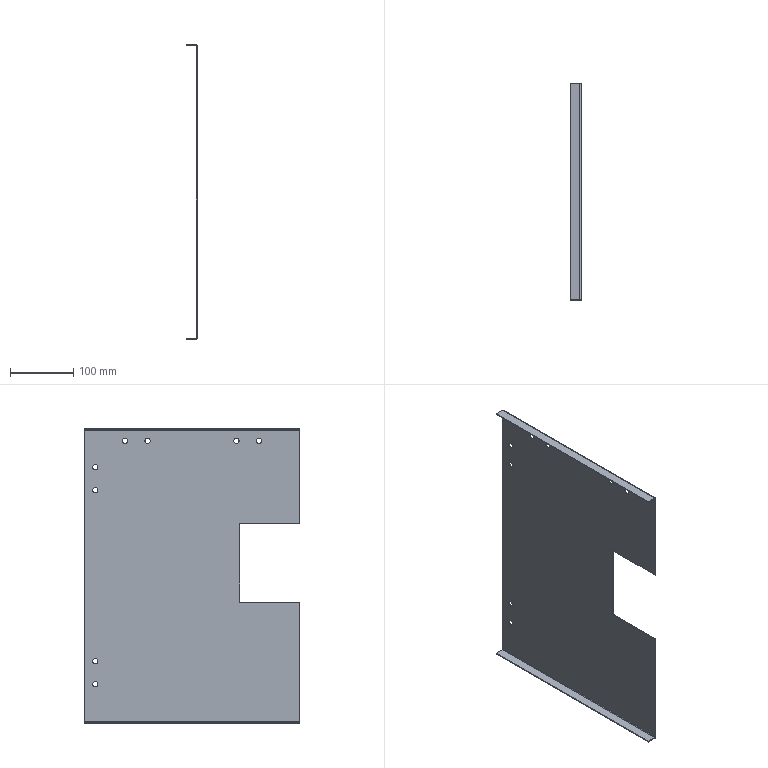Part | SolidWorks | features BaseBody 1 | 1 solid | 34 faces | box 16.5 x 340 x 464 mm | volume 232938 mm3 | cylinder 20 | plane 14 | commonest cylinder face diameters 8.5 x16 1.473 x2 4.473 x2
STEP:
#1=CARTESIAN_POINT('',(0.,276.,-13.25));
#2=VERTEX_POINT('',#1);
#3=CARTESIAN_POINT('',(0.,276.,-21.75));
#4=VERTEX_POINT('',#3);
#5=CARTESIAN_POINT('',(0.,276.,-17.5));
#6=DIRECTION('',(1.,0.,0.));
#7=DIRECTION('',(0.,0.,-1.));
#8=AXIS2_PLACEMENT_3D('',#5,#6,#7);
#9=CIRCLE('',#8,4.25);
#10=EDGE_CURVE('',#2,#4,#9,.T.);
#11=ORIENTED_EDGE('',*,*,#10,.F.);
#12=CARTESIAN_POINT('',(1.5,276.,-13.25));
#13=VERTEX_POINT('',#12);
#14=CARTESIAN_POINT('',(-8.5,276.,-13.25));
#15=DIRECTION('',(1.,0.,0.));
#16=VECTOR('',#15,1000.);
#17=LINE('',#14,#16);
#18=EDGE_CURVE('',#2,#13,#17,.T.);
#19=ORIENTED_EDGE('',*,*,#18,.T.);
#20=CARTESIAN_POINT('',(1.5,276.,-21.75));
#21=VERTEX_POINT('',#20);
#22=CARTESIAN_POINT('',(1.5,276.,-17.5));
#23=DIRECTION('',(-1.,0.,0.));
#24=DIRECTION('',(0.,0.,-1.));
#25=AXIS2_PLACEMENT_3D('',#22,#23,#24);
#26=CIRCLE('',#25,4.25);
#27=EDGE_CURVE('',#21,#13,#26,.T.);
#28=ORIENTED_EDGE('',*,*,#27,.F.);
#29=CARTESIAN_POINT('',(-8.5,276.,-21.75));
#30=DIRECTION('',(1.,0.,0.));
#31=VECTOR('',#30,1000.);
#32=LINE('',#29,#31);
#33=EDGE_CURVE('',#4,#21,#32,.T.);
#34=ORIENTED_EDGE('',*,*,#33,.F.);
#35=EDGE_LOOP('',(#11,#19,#28,#34));
#36=FACE_OUTER_BOUND('',#35,.T.);
#37=CARTESIAN_POINT('',(-8.5,276.,-17.5));
#38=DIRECTION('',(1.,0.,0.));
#39=DIRECTION('',(0.,0.,-1.));
#40=AXIS2_PLACEMENT_3D('',#37,#38,#39);
#41=CYLINDRICAL_SURFACE('',#40,4.25);
#42=ADVANCED_FACE('',(#36),#41,.F.);
#43=CARTESIAN_POINT('',(0.,322.5,-396.75));
#44=VERTEX_POINT('',#43);
#45=CARTESIAN_POINT('',(0.,322.5,-405.25));
#46=VERTEX_POINT('',#45);
#47=CARTESIAN_POINT('',(0.,322.5,-401.));
#48=DIRECTION('',(1.,0.,0.));
#49=DIRECTION('',(0.,0.,-1.));
#50=AXIS2_PLACEMENT_3D('',#47,#48,#49);
#51=CIRCLE('',#50,4.25);
#52=EDGE_CURVE('',#44,#46,#51,.T.);
#53=ORIENTED_EDGE('',*,*,#52,.F.);
#54=CARTESIAN_POINT('',(1.5,322.5,-396.75));
#55=VERTEX_POINT('',#54);
#56=CARTESIAN_POINT('',(-8.5,322.5,-396.75));
#57=DIRECTION('',(1.,0.,0.));
#58=VECTOR('',#57,1000.);
#59=LINE('',#56,#58);
#60=EDGE_CURVE('',#44,#55,#59,.T.);
#61=ORIENTED_EDGE('',*,*,#60,.T.);
#62=CARTESIAN_POINT('',(1.5,322.5,-405.25));
#63=VERTEX_POINT('',#62);
#64=CARTESIAN_POINT('',(1.5,322.5,-401.));
#65=DIRECTION('',(-1.,0.,0.));
#66=DIRECTION('',(0.,0.,-1.));
#67=AXIS2_PLACEMENT_3D('',#64,#65,#66);
#68=CIRCLE('',#67,4.25);
#69=EDGE_CURVE('',#63,#55,#68,.T.);
#70=ORIENTED_EDGE('',*,*,#69,.F.);
#71=CARTESIAN_POINT('',(-8.5,322.5,-405.25));
#72=DIRECTION('',(1.,0.,0.));
#73=VECTOR('',#72,1000.);
#74=LINE('',#71,#73);
#75=EDGE_CURVE('',#46,#63,#74,.T.);
#76=ORIENTED_EDGE('',*,*,#75,.F.);
#77=EDGE_LOOP('',(#53,#61,#70,#76));
#78=FACE_OUTER_BOUND('',#77,.T.);
#79=CARTESIAN_POINT('',(-8.5,322.5,-401.));
#80=DIRECTION('',(1.,0.,0.));
#81=DIRECTION('',(0.,0.,-1.));
#82=AXIS2_PLACEMENT_3D('',#79,#80,#81);
#83=CYLINDRICAL_SURFACE('',#82,4.25);
#84=ADVANCED_FACE('',(#78),#83,.F.);
#85=CARTESIAN_POINT('',(0.,322.5,-360.75));
#86=VERTEX_POINT('',#85);
#87=CARTESIAN_POINT('',(0.,322.5,-369.25));
#88=VERTEX_POINT('',#87);
#89=CARTESIAN_POINT('',(0.,322.5,-365.));
#90=DIRECTION('',(1.,0.,0.));
#91=DIRECTION('',(0.,0.,-1.));
#92=AXIS2_PLACEMENT_3D('',#89,#90,#91);
#93=CIRCLE('',#92,4.25);
#94=EDGE_CURVE('',#86,#88,#93,.T.);
#95=ORIENTED_EDGE('',*,*,#94,.F.);
#96=CARTESIAN_POINT('',(1.5,322.5,-360.75));
#97=VERTEX_POINT('',#96);
#98=CARTESIAN_POINT('',(-8.5,322.5,-360.75));
#99=DIRECTION('',(1.,0.,0.));
#100=VECTOR('',#99,1000.);
#101=LINE('',#98,#100);
#102=EDGE_CURVE('',#86,#97,#101,.T.);
#103=ORIENTED_EDGE('',*,*,#102,.T.);
#104=CARTESIAN_POINT('',(1.5,322.5,-369.25));
#105=VERTEX_POINT('',#104);
#106=CARTESIAN_POINT('',(1.5,322.5,-365.));
#107=DIRECTION('',(-1.,0.,0.));
#108=DIRECTION('',(0.,0.,-1.));
#109=AXIS2_PLACEMENT_3D('',#106,#107,#108);
#110=CIRCLE('',#109,4.25);
#111=EDGE_CURVE('',#105,#97,#110,.T.);
#112=ORIENTED_EDGE('',*,*,#111,.F.);
#113=CARTESIAN_POINT('',(-8.5,322.5,-369.25));
#114=DIRECTION('',(1.,0.,0.));
#115=VECTOR('',#114,1000.);
#116=LINE('',#113,#115);
#117=EDGE_CURVE('',#88,#105,#116,.T.);
#118=ORIENTED_EDGE('',*,*,#117,.F.);
#119=EDGE_LOOP('',(#95,#103,#112,#118));
#120=FACE_OUTER_BOUND('',#119,.T.);
#121=CARTESIAN_POINT('',(-8.5,322.5,-365.));
#122=DIRECTION('',(1.,0.,0.));
#123=DIRECTION('',(0.,0.,-1.));
#124=AXIS2_PLACEMENT_3D('',#121,#122,#123);
#125=CYLINDRICAL_SURFACE('',#124,4.25);
#126=ADVANCED_FACE('',(#120),#125,.F.);
#127=CARTESIAN_POINT('',(0.,322.5,-54.75));
#128=VERTEX_POINT('',#127);
#129=CARTESIAN_POINT('',(0.,322.5,-63.25));
#130=VERTEX_POINT('',#129);
#131=CARTESIAN_POINT('',(0.,322.5,-59.));
#132=DIRECTION('',(1.,0.,0.));
#133=DIRECTION('',(0.,0.,-1.));
#134=AXIS2_PLACEMENT_3D('',#131,#132,#133);
#135=CIRCLE('',#134,4.25);
#136=EDGE_CURVE('',#128,#130,#135,.T.);
#137=ORIENTED_EDGE('',*,*,#136,.F.);
#138=CARTESIAN_POINT('',(1.5,322.5,-54.75));
#139=VERTEX_POINT('',#138);
#140=CARTESIAN_POINT('',(-8.5,322.5,-54.75));
#141=DIRECTION('',(1.,0.,0.));
#142=VECTOR('',#141,1000.);
#143=LINE('',#140,#142);
#144=EDGE_CURVE('',#128,#139,#143,.T.);
#145=ORIENTED_EDGE('',*,*,#144,.T.);
#146=CARTESIAN_POINT('',(1.5,322.5,-63.25));
#147=VERTEX_POINT('',#146);
#148=CARTESIAN_POINT('',(1.5,322.5,-59.));
#149=DIRECTION('',(-1.,0.,0.));
#150=DIRECTION('',(0.,0.,-1.));
#151=AXIS2_PLACEMENT_3D('',#148,#149,#150);
#152=CIRCLE('',#151,4.25);
#153=EDGE_CURVE('',#147,#139,#152,.T.);
#154=ORIENTED_EDGE('',*,*,#153,.F.);
#155=CARTESIAN_POINT('',(-8.5,322.5,-63.25));
#156=DIRECTION('',(1.,0.,0.));
#157=VECTOR('',#156,1000.);
#158=LINE('',#155,#157);
#159=EDGE_CURVE('',#130,#147,#158,.T.);
#160=ORIENTED_EDGE('',*,*,#159,.F.);
#161=EDGE_LOOP('',(#137,#145,#154,#160));
#162=FACE_OUTER_BOUND('',#161,.T.);
#163=CARTESIAN_POINT('',(-8.5,322.5,-59.));
#164=DIRECTION('',(1.,0.,0.));
#165=DIRECTION('',(0.,0.,-1.));
#166=AXIS2_PLACEMENT_3D('',#163,#164,#165);
#167=CYLINDRICAL_SURFACE('',#166,4.25);
#168=ADVANCED_FACE('',(#162),#167,.F.);
#169=CARTESIAN_POINT('',(0.,322.5,-90.75));
#170=VERTEX_POINT('',#169);
#171=CARTESIAN_POINT('',(0.,322.5,-99.25));
#172=VERTEX_POINT('',#171);
#173=CARTESIAN_POINT('',(0.,322.5,-95.));
#174=DIRECTION('',(1.,0.,0.));
#175=DIRECTION('',(0.,0.,-1.));
#176=AXIS2_PLACEMENT_3D('',#173,#174,#175);
#177=CIRCLE('',#176,4.25);
#178=EDGE_CURVE('',#170,#172,#177,.T.);
#179=ORIENTED_EDGE('',*,*,#178,.F.);
#180=CARTESIAN_POINT('',(1.5,322.5,-90.75));
#181=VERTEX_POINT('',#180);
#182=CARTESIAN_POINT('',(-8.5,322.5,-90.75));
#183=DIRECTION('',(1.,0.,0.));
#184=VECTOR('',#183,1000.);
#185=LINE('',#182,#184);
#186=EDGE_CURVE('',#170,#181,#185,.T.);
#187=ORIENTED_EDGE('',*,*,#186,.T.);
#188=CARTESIAN_POINT('',(1.5,322.5,-99.25));
#189=VERTEX_POINT('',#188);
#190=CARTESIAN_POINT('',(1.5,322.5,-95.));
#191=DIRECTION('',(-1.,0.,0.));
#192=DIRECTION('',(0.,0.,-1.));
#193=AXIS2_PLACEMENT_3D('',#190,#191,#192);
#194=CIRCLE('',#193,4.25);
#195=EDGE_CURVE('',#189,#181,#194,.T.);
#196=ORIENTED_EDGE('',*,*,#195,.F.);
#197=CARTESIAN_POINT('',(-8.5,322.5,-99.25));
#198=DIRECTION('',(1.,0.,0.));
#199=VECTOR('',#198,1000.);
#200=LINE('',#197,#199);
#201=EDGE_CURVE('',#172,#189,#200,.T.);
#202=ORIENTED_EDGE('',*,*,#201,.F.);
#203=EDGE_LOOP('',(#179,#187,#196,#202));
#204=FACE_OUTER_BOUND('',#203,.T.);
#205=CARTESIAN_POINT('',(-8.5,322.5,-95.));
#206=DIRECTION('',(1.,0.,0.));
#207=DIRECTION('',(0.,0.,-1.));
#208=AXIS2_PLACEMENT_3D('',#205,#206,#207);
#209=CYLINDRICAL_SURFACE('',#208,4.25);
#210=ADVANCED_FACE('',(#204),#209,.F.);
#211=CARTESIAN_POINT('',(0.,64.,-13.25));
#212=VERTEX_POINT('',#211);
#213=CARTESIAN_POINT('',(0.,64.,-21.75));
#214=VERTEX_POINT('',#213);
#215=CARTESIAN_POINT('',(0.,64.,-17.5));
#216=DIRECTION('',(1.,0.,0.));
#217=DIRECTION('',(0.,0.,-1.));
#218=AXIS2_PLACEMENT_3D('',#215,#216,#217);
#219=CIRCLE('',#218,4.25);
#220=EDGE_CURVE('',#212,#214,#219,.T.);
#221=ORIENTED_EDGE('',*,*,#220,.F.);
#222=CARTESIAN_POINT('',(1.5,64.,-13.25));
#223=VERTEX_POINT('',#222);
#224=CARTESIAN_POINT('',(-8.5,64.,-13.25));
#225=DIRECTION('',(1.,0.,0.));
#226=VECTOR('',#225,1000.);
#227=LINE('',#224,#226);
#228=EDGE_CURVE('',#212,#223,#227,.T.);
#229=ORIENTED_EDGE('',*,*,#228,.T.);
#230=CARTESIAN_POINT('',(1.5,64.,-21.75));
#231=VERTEX_POINT('',#230);
#232=CARTESIAN_POINT('',(1.5,64.,-17.5));
#233=DIRECTION('',(-1.,0.,0.));
#234=DIRECTION('',(0.,0.,-1.));
#235=AXIS2_PLACEMENT_3D('',#232,#233,#234);
#236=CIRCLE('',#235,4.25);
#237=EDGE_CURVE('',#231,#223,#236,.T.);
#238=ORIENTED_EDGE('',*,*,#237,.F.);
#239=CARTESIAN_POINT('',(-8.5,64.,-21.75));
#240=DIRECTION('',(1.,0.,0.));
#241=VECTOR('',#240,1000.);
#242=LINE('',#239,#241);
#243=EDGE_CURVE('',#214,#231,#242,.T.);
#244=ORIENTED_EDGE('',*,*,#243,.F.);
#245=EDGE_LOOP('',(#221,#229,#238,#244));
#246=FACE_OUTER_BOUND('',#245,.T.);
#247=CARTESIAN_POINT('',(-8.5,64.,-17.5));
#248=DIRECTION('',(1.,0.,0.));
#249=DIRECTION('',(0.,0.,-1.));
#250=AXIS2_PLACEMENT_3D('',#247,#248,#249);
#251=CYLINDRICAL_SURFACE('',#250,4.25);
#252=ADVANCED_FACE('',(#246),#251,.F.);
#253=CARTESIAN_POINT('',(0.,100.,-13.25));
#254=VERTEX_POINT('',#253);
#255=CARTESIAN_POINT('',(0.,100.,-21.75));
#256=VERTEX_POINT('',#255);
#257=CARTESIAN_POINT('',(0.,100.,-17.5));
#258=DIRECTION('',(1.,0.,0.));
#259=DIRECTION('',(0.,0.,-1.));
#260=AXIS2_PLACEMENT_3D('',#257,#258,#259);
#261=CIRCLE('',#260,4.25);
#262=EDGE_CURVE('',#254,#256,#261,.T.);
#263=ORIENTED_EDGE('',*,*,#262,.F.);
#264=CARTESIAN_POINT('',(1.5,100.,-13.25));
#265=VERTEX_POINT('',#264);
#266=CARTESIAN_POINT('',(-8.5,100.,-13.25));
#267=DIRECTION('',(1.,0.,0.));
#268=VECTOR('',#267,1000.);
#269=LINE('',#266,#268);
#270=EDGE_CURVE('',#254,#265,#269,.T.);
#271=ORIENTED_EDGE('',*,*,#270,.T.);
#272=CARTESIAN_POINT('',(1.5,100.,-21.75));
#273=VERTEX_POINT('',#272);
#274=CARTESIAN_POINT('',(1.5,100.,-17.5));
#275=DIRECTION('',(-1.,0.,0.));
#276=DIRECTION('',(0.,0.,-1.));
#277=AXIS2_PLACEMENT_3D('',#274,#275,#276);
#278=CIRCLE('',#277,4.25);
#279=EDGE_CURVE('',#273,#265,#278,.T.);
#280=ORIENTED_EDGE('',*,*,#279,.F.);
#281=CARTESIAN_POINT('',(-8.5,100.,-21.75));
#282=DIRECTION('',(1.,0.,0.));
#283=VECTOR('',#282,1000.);
#284=LINE('',#281,#283);
#285=EDGE_CURVE('',#256,#273,#284,.T.);
#286=ORIENTED_EDGE('',*,*,#285,.F.);
#287=EDGE_LOOP('',(#263,#271,#280,#286));
#288=FACE_OUTER_BOUND('',#287,.T.);
#289=CARTESIAN_POINT('',(-8.5,100.,-17.5));
#290=DIRECTION('',(1.,0.,0.));
#291=DIRECTION('',(0.,0.,-1.));
#292=AXIS2_PLACEMENT_3D('',#289,#290,#291);
#293=CYLINDRICAL_SURFACE('',#292,4.25);
#294=ADVANCED_FACE('',(#288),#293,.F.);
#295=CARTESIAN_POINT('',(0.,240.,-13.25));
#296=VERTEX_POINT('',#295);
#297=CARTESIAN_POINT('',(0.,240.,-21.75));
#298=VERTEX_POINT('',#297);
#299=CARTESIAN_POINT('',(0.,240.,-17.5));
#300=DIRECTION('',(1.,0.,0.));
#301=DIRECTION('',(0.,0.,-1.));
#302=AXIS2_PLACEMENT_3D('',#299,#300,#301);
#303=CIRCLE('',#302,4.25);
#304=EDGE_CURVE('',#296,#298,#303,.T.);
#305=ORIENTED_EDGE('',*,*,#304,.F.);
#306=CARTESIAN_POINT('',(1.5,240.,-13.25));
#307=VERTEX_POINT('',#306);
#308=CARTESIAN_POINT('',(-8.5,240.,-13.25));
#309=DIRECTION('',(1.,0.,0.));
#310=VECTOR('',#309,1000.);
#311=LINE('',#308,#310);
#312=EDGE_CURVE('',#296,#307,#311,.T.);
#313=ORIENTED_EDGE('',*,*,#312,.T.);
#314=CARTESIAN_POINT('',(1.5,240.,-21.75));
#315=VERTEX_POINT('',#314);
#316=CARTESIAN_POINT('',(1.5,240.,-17.5));
#317=DIRECTION('',(-1.,0.,0.));
#318=DIRECTION('',(0.,0.,-1.));
#319=AXIS2_PLACEMENT_3D('',#316,#317,#318);
#320=CIRCLE('',#319,4.25);
#321=EDGE_CURVE('',#315,#307,#320,.T.);
#322=ORIENTED_EDGE('',*,*,#321,.F.);
#323=CARTESIAN_POINT('',(-8.5,240.,-21.75));
#324=DIRECTION('',(1.,0.,0.));
#325=VECTOR('',#324,1000.);
#326=LINE('',#323,#325);
#327=EDGE_CURVE('',#298,#315,#326,.T.);
#328=ORIENTED_EDGE('',*,*,#327,.F.);
#329=EDGE_LOOP('',(#305,#313,#322,#328));
#330=FACE_OUTER_BOUND('',#329,.T.);
#331=CARTESIAN_POINT('',(-8.5,240.,-17.5));
#332=DIRECTION('',(1.,0.,0.));
#333=DIRECTION('',(0.,0.,-1.));
#334=AXIS2_PLACEMENT_3D('',#331,#332,#333);
#335=CYLINDRICAL_SURFACE('',#334,4.25);
#336=ADVANCED_FACE('',(#330),#335,.F.);
#337=CARTESIAN_POINT('',(0.,276.,-17.5));
#338=DIRECTION('',(1.,0.,0.));
#339=DIRECTION('',(0.,0.,-1.));
#340=AXIS2_PLACEMENT_3D('',#337,#338,#339);
#341=CIRCLE('',#340,4.25);
#342=EDGE_CURVE('',#4,#2,#341,.T.);
#343=ORIENTED_EDGE('',*,*,#342,.T.);
#344=ORIENTED_EDGE('',*,*,#10,.T.);
#345=EDGE_LOOP('',(#343,#344));
#346=FACE_BOUND('',#345,.T.);
#347=CARTESIAN_POINT('',(0.,322.5,-401.));
#348=DIRECTION('',(1.,0.,0.));
#349=DIRECTION('',(0.,0.,-1.));
#350=AXIS2_PLACEMENT_3D('',#347,#348,#349);
#351=CIRCLE('',#350,4.25);
#352=EDGE_CURVE('',#46,#44,#351,.T.);
#353=ORIENTED_EDGE('',*,*,#352,.T.);
#354=ORIENTED_EDGE('',*,*,#52,.T.);
#355=EDGE_LOOP('',(#353,#354));
#356=FACE_BOUND('',#355,.T.);
#357=CARTESIAN_POINT('',(0.,322.5,-365.));
#358=DIRECTION('',(1.,0.,0.));
#359=DIRECTION('',(0.,0.,-1.));
#360=AXIS2_PLACEMENT_3D('',#357,#358,#359);
#361=CIRCLE('',#360,4.25);
#362=EDGE_CURVE('',#88,#86,#361,.T.);
#363=ORIENTED_EDGE('',*,*,#362,.T.);
#364=ORIENTED_EDGE('',*,*,#94,.T.);
#365=EDGE_LOOP('',(#363,#364));
#366=FACE_BOUND('',#365,.T.);
#367=CARTESIAN_POINT('',(0.,322.5,-59.));
#368=DIRECTION('',(1.,0.,0.));
#369=DIRECTION('',(0.,0.,-1.));
#370=AXIS2_PLACEMENT_3D('',#367,#368,#369);
#371=CIRCLE('',#370,4.25);
#372=EDGE_CURVE('',#130,#128,#371,.T.);
#373=ORIENTED_EDGE('',*,*,#372,.T.);
#374=ORIENTED_EDGE('',*,*,#136,.T.);
#375=EDGE_LOOP('',(#373,#374));
#376=FACE_BOUND('',#375,.T.);
#377=CARTESIAN_POINT('',(0.,322.5,-95.));
#378=DIRECTION('',(1.,0.,0.));
#379=DIRECTION('',(0.,0.,-1.));
#380=AXIS2_PLACEMENT_3D('',#377,#378,#379);
#381=CIRCLE('',#380,4.25);
#382=EDGE_CURVE('',#172,#170,#381,.T.);
#383=ORIENTED_EDGE('',*,*,#382,.T.);
#384=ORIENTED_EDGE('',*,*,#178,.T.);
#385=EDGE_LOOP('',(#383,#384));
#386=FACE_BOUND('',#385,.T.);
#387=CARTESIAN_POINT('',(0.,64.,-17.5));
#388=DIRECTION('',(1.,0.,0.));
#389=DIRECTION('',(0.,0.,-1.));
#390=AXIS2_PLACEMENT_3D('',#387,#388,#389);
#391=CIRCLE('',#390,4.25);
#392=EDGE_CURVE('',#214,#212,#391,.T.);
#393=ORIENTED_EDGE('',*,*,#392,.T.);
#394=ORIENTED_EDGE('',*,*,#220,.T.);
#395=EDGE_LOOP('',(#393,#394));
#396=FACE_BOUND('',#395,.T.);
#397=CARTESIAN_POINT('',(0.,100.,-17.5));
#398=DIRECTION('',(1.,0.,0.));
#399=DIRECTION('',(0.,0.,-1.));
#400=AXIS2_PLACEMENT_3D('',#397,#398,#399);
#401=CIRCLE('',#400,4.25);
#402=EDGE_CURVE('',#256,#254,#401,.T.);
#403=ORIENTED_EDGE('',*,*,#402,.T.);
#404=ORIENTED_EDGE('',*,*,#262,.T.);
#405=EDGE_LOOP('',(#403,#404));
#406=FACE_BOUND('',#405,.T.);
#407=CARTESIAN_POINT('',(0.,240.,-17.5));
#408=DIRECTION('',(1.,0.,0.));
#409=DIRECTION('',(0.,0.,-1.));
#410=AXIS2_PLACEMENT_3D('',#407,#408,#409);
#411=CIRCLE('',#410,4.25);
#412=EDGE_CURVE('',#298,#296,#411,.T.);
#413=ORIENTED_EDGE('',*,*,#412,.T.);
#414=ORIENTED_EDGE('',*,*,#304,.T.);
#415=EDGE_LOOP('',(#413,#414));
#416=FACE_BOUND('',#415,.T.);
#417=CARTESIAN_POINT('',(0.,0.,-271.737));
#418=VERTEX_POINT('',#417);
#419=CARTESIAN_POINT('',(0.,95.,-271.737));
#420=VERTEX_POINT('',#419);
#421=CARTESIAN_POINT('',(0.,340.,-271.737));
#422=DIRECTION('',(0.,1.,0.));
#423=VECTOR('',#422,1000.);
#424=LINE('',#421,#423);
#425=EDGE_CURVE('',#418,#420,#424,.T.);
#426=ORIENTED_EDGE('',*,*,#425,.T.);
#427=CARTESIAN_POINT('',(0.,95.,-147.737));
#428=VERTEX_POINT('',#427);
#429=CARTESIAN_POINT('',(0.,95.,0.));
#430=DIRECTION('',(0.,0.,1.));
#431=VECTOR('',#430,1000.);
#432=LINE('',#429,#431);
#433=EDGE_CURVE('',#420,#428,#432,.T.);
#434=ORIENTED_EDGE('',*,*,#433,.T.);
#435=CARTESIAN_POINT('',(0.,0.,-147.737));
#436=VERTEX_POINT('',#435);
#437=CARTESIAN_POINT('',(0.,340.,-147.737));
#438=DIRECTION('',(0.,-1.,0.));
#439=VECTOR('',#438,1000.);
#440=LINE('',#437,#439);
#441=EDGE_CURVE('',#428,#436,#440,.T.);
#442=ORIENTED_EDGE('',*,*,#441,.T.);
#443=CARTESIAN_POINT('',(0.,0.,-0.7366));
#444=VERTEX_POINT('',#443);
#445=CARTESIAN_POINT('',(0.,0.,0.));
#446=DIRECTION('',(0.,0.,1.));
#447=VECTOR('',#446,1000.);
#448=LINE('',#445,#447);
#449=EDGE_CURVE('',#436,#444,#448,.T.);
#450=ORIENTED_EDGE('',*,*,#449,.T.);
#451=CARTESIAN_POINT('',(0.,340.,-0.7366));
#452=VERTEX_POINT('',#451);
#453=CARTESIAN_POINT('',(0.,340.,-0.7366));
#454=DIRECTION('',(0.,1.,0.));
#455=VECTOR('',#454,1000.);
#456=LINE('',#453,#455);
#457=EDGE_CURVE('',#444,#452,#456,.T.);
#458=ORIENTED_EDGE('',*,*,#457,.T.);
#459=CARTESIAN_POINT('',(0.,340.,-460.263));
#460=VERTEX_POINT('',#459);
#461=CARTESIAN_POINT('',(0.,340.,0.));
#462=DIRECTION('',(0.,0.,-1.));
#463=VECTOR('',#462,1000.);
#464=LINE('',#461,#463);
#465=EDGE_CURVE('',#452,#460,#464,.T.);
#466=ORIENTED_EDGE('',*,*,#465,.T.);
#467=CARTESIAN_POINT('',(0.,0.,-460.263));
#468=VERTEX_POINT('',#467);
#469=CARTESIAN_POINT('',(0.,340.,-460.263));
#470=DIRECTION('',(0.,-1.,0.));
#471=VECTOR('',#470,1000.);
#472=LINE('',#469,#471);
#473=EDGE_CURVE('',#460,#468,#472,.T.);
#474=ORIENTED_EDGE('',*,*,#473,.T.);
#475=CARTESIAN_POINT('',(0.,0.,0.));
#476=DIRECTION('',(0.,0.,1.));
#477=VECTOR('',#476,1000.);
#478=LINE('',#475,#477);
#479=EDGE_CURVE('',#468,#418,#478,.T.);
#480=ORIENTED_EDGE('',*,*,#479,.T.);
#481=EDGE_LOOP('',(#426,#434,#442,#450,#458,#466,#474,#480));
#482=FACE_OUTER_BOUND('',#481,.T.);
#483=CARTESIAN_POINT('',(0.,340.,0.));
#484=DIRECTION('',(-1.,0.,0.));
#485=DIRECTION('',(0.,0.,1.));
#486=AXIS2_PLACEMENT_3D('',#483,#484,#485);
#487=PLANE('',#486);
#488=ADVANCED_FACE('',(#346,#356,#366,#376,#386,#396,#406,#416,#482),#487,.T.);
#489=ORIENTED_EDGE('',*,*,#18,.F.);
#490=ORIENTED_EDGE('',*,*,#342,.F.);
#491=ORIENTED_EDGE('',*,*,#33,.T.);
#492=CARTESIAN_POINT('',(1.5,276.,-17.5));
#493=DIRECTION('',(-1.,0.,0.));
#494=DIRECTION('',(0.,0.,-1.));
#495=AXIS2_PLACEMENT_3D('',#492,#493,#494);
#496=CIRCLE('',#495,4.25);
#497=EDGE_CURVE('',#13,#21,#496,.T.);
#498=ORIENTED_EDGE('',*,*,#497,.F.);
#499=EDGE_LOOP('',(#489,#490,#491,#498));
#500=FACE_OUTER_BOUND('',#499,.T.);
#501=CARTESIAN_POINT('',(-8.5,276.,-17.5));
#502=DIRECTION('',(1.,0.,0.));
#503=DIRECTION('',(0.,0.,-1.));
#504=AXIS2_PLACEMENT_3D('',#501,#502,#503);
#505=CYLINDRICAL_SURFACE('',#504,4.25);
#506=ADVANCED_FACE('',(#500),#505,.F.);
#507=ORIENTED_EDGE('',*,*,#60,.F.);
#508=ORIENTED_EDGE('',*,*,#352,.F.);
#509=ORIENTED_EDGE('',*,*,#75,.T.);
#510=CARTESIAN_POINT('',(1.5,322.5,-401.));
#511=DIRECTION('',(-1.,0.,0.));
#512=DIRECTION('',(0.,0.,-1.));
#513=AXIS2_PLACEMENT_3D('',#510,#511,#512);
#514=CIRCLE('',#513,4.25);
#515=EDGE_CURVE('',#55,#63,#514,.T.);
#516=ORIENTED_EDGE('',*,*,#515,.F.);
#517=EDGE_LOOP('',(#507,#508,#509,#516));
#518=FACE_OUTER_BOUND('',#517,.T.);
#519=CARTESIAN_POINT('',(-8.5,322.5,-401.));
#520=DIRECTION('',(1.,0.,0.));
#521=DIRECTION('',(0.,0.,-1.));
#522=AXIS2_PLACEMENT_3D('',#519,#520,#521);
#523=CYLINDRICAL_SURFACE('',#522,4.25);
#524=ADVANCED_FACE('',(#518),#523,.F.);
#525=ORIENTED_EDGE('',*,*,#102,.F.);
#526=ORIENTED_EDGE('',*,*,#362,.F.);
#527=ORIENTED_EDGE('',*,*,#117,.T.);
#528=CARTESIAN_POINT('',(1.5,322.5,-365.));
#529=DIRECTION('',(-1.,0.,0.));
#530=DIRECTION('',(0.,0.,-1.));
#531=AXIS2_PLACEMENT_3D('',#528,#529,#530);
#532=CIRCLE('',#531,4.25);
#533=EDGE_CURVE('',#97,#105,#532,.T.);
#534=ORIENTED_EDGE('',*,*,#533,.F.);
#535=EDGE_LOOP('',(#525,#526,#527,#534));
#536=FACE_OUTER_BOUND('',#535,.T.);
#537=CARTESIAN_POINT('',(-8.5,322.5,-365.));
#538=DIRECTION('',(1.,0.,0.));
#539=DIRECTION('',(0.,0.,-1.));
#540=AXIS2_PLACEMENT_3D('',#537,#538,#539);
#541=CYLINDRICAL_SURFACE('',#540,4.25);
#542=ADVANCED_FACE('',(#536),#541,.F.);
#543=ORIENTED_EDGE('',*,*,#144,.F.);
#544=ORIENTED_EDGE('',*,*,#372,.F.);
#545=ORIENTED_EDGE('',*,*,#159,.T.);
#546=CARTESIAN_POINT('',(1.5,322.5,-59.));
#547=DIRECTION('',(-1.,0.,0.));
#548=DIRECTION('',(0.,0.,-1.));
#549=AXIS2_PLACEMENT_3D('',#546,#547,#548);
#550=CIRCLE('',#549,4.25);
#551=EDGE_CURVE('',#139,#147,#550,.T.);
#552=ORIENTED_EDGE('',*,*,#551,.F.);
#553=EDGE_LOOP('',(#543,#544,#545,#552));
#554=FACE_OUTER_BOUND('',#553,.T.);
#555=CARTESIAN_POINT('',(-8.5,322.5,-59.));
#556=DIRECTION('',(1.,0.,0.));
#557=DIRECTION('',(0.,0.,-1.));
#558=AXIS2_PLACEMENT_3D('',#555,#556,#557);
#559=CYLINDRICAL_SURFACE('',#558,4.25);
#560=ADVANCED_FACE('',(#554),#559,.F.);
#561=ORIENTED_EDGE('',*,*,#186,.F.);
#562=ORIENTED_EDGE('',*,*,#382,.F.);
#563=ORIENTED_EDGE('',*,*,#201,.T.);
#564=CARTESIAN_POINT('',(1.5,322.5,-95.));
#565=DIRECTION('',(-1.,0.,0.));
#566=DIRECTION('',(0.,0.,-1.));
#567=AXIS2_PLACEMENT_3D('',#564,#565,#566);
#568=CIRCLE('',#567,4.25);
#569=EDGE_CURVE('',#181,#189,#568,.T.);
#570=ORIENTED_EDGE('',*,*,#569,.F.);
#571=EDGE_LOOP('',(#561,#562,#563,#570));
#572=FACE_OUTER_BOUND('',#571,.T.);
#573=CARTESIAN_POINT('',(-8.5,322.5,-95.));
#574=DIRECTION('',(1.,0.,0.));
#575=DIRECTION('',(0.,0.,-1.));
#576=AXIS2_PLACEMENT_3D('',#573,#574,#575);
#577=CYLINDRICAL_SURFACE('',#576,4.25);
#578=ADVANCED_FACE('',(#572),#577,.F.);
#579=ORIENTED_EDGE('',*,*,#228,.F.);
#580=ORIENTED_EDGE('',*,*,#392,.F.);
#581=ORIENTED_EDGE('',*,*,#243,.T.);
#582=CARTESIAN_POINT('',(1.5,64.,-17.5));
#583=DIRECTION('',(-1.,0.,0.));
#584=DIRECTION('',(0.,0.,-1.));
#585=AXIS2_PLACEMENT_3D('',#582,#583,#584);
#586=CIRCLE('',#585,4.25);
#587=EDGE_CURVE('',#223,#231,#586,.T.);
#588=ORIENTED_EDGE('',*,*,#587,.F.);
#589=EDGE_LOOP('',(#579,#580,#581,#588));
#590=FACE_OUTER_BOUND('',#589,.T.);
#591=CARTESIAN_POINT('',(-8.5,64.,-17.5));
#592=DIRECTION('',(1.,0.,0.));
#593=DIRECTION('',(0.,0.,-1.));
#594=AXIS2_PLACEMENT_3D('',#591,#592,#593);
#595=CYLINDRICAL_SURFACE('',#594,4.25);
#596=ADVANCED_FACE('',(#590),#595,.F.);
#597=ORIENTED_EDGE('',*,*,#270,.F.);
#598=ORIENTED_EDGE('',*,*,#402,.F.);
#599=ORIENTED_EDGE('',*,*,#285,.T.);
#600=CARTESIAN_POINT('',(1.5,100.,-17.5));
#601=DIRECTION('',(-1.,0.,0.));
#602=DIRECTION('',(0.,0.,-1.));
#603=AXIS2_PLACEMENT_3D('',#600,#601,#602);
#604=CIRCLE('',#603,4.25);
#605=EDGE_CURVE('',#265,#273,#604,.T.);
#606=ORIENTED_EDGE('',*,*,#605,.F.);
#607=EDGE_LOOP('',(#597,#598,#599,#606));
#608=FACE_OUTER_BOUND('',#607,.T.);
#609=CARTESIAN_POINT('',(-8.5,100.,-17.5));
#610=DIRECTION('',(1.,0.,0.));
#611=DIRECTION('',(0.,0.,-1.));
#612=AXIS2_PLACEMENT_3D('',#609,#610,#611);
#613=CYLINDRICAL_SURFACE('',#612,4.25);
#614=ADVANCED_FACE('',(#608),#613,.F.);
#615=ORIENTED_EDGE('',*,*,#312,.F.);
#616=ORIENTED_EDGE('',*,*,#412,.F.);
#617=ORIENTED_EDGE('',*,*,#327,.T.);
#618=CARTESIAN_POINT('',(1.5,240.,-17.5));
#619=DIRECTION('',(-1.,0.,0.));
#620=DIRECTION('',(0.,0.,-1.));
#621=AXIS2_PLACEMENT_3D('',#618,#619,#620);
#622=CIRCLE('',#621,4.25);
#623=EDGE_CURVE('',#307,#315,#622,.T.);
#624=ORIENTED_EDGE('',*,*,#623,.F.);
#625=EDGE_LOOP('',(#615,#616,#617,#624));
#626=FACE_OUTER_BOUND('',#625,.T.);
#627=CARTESIAN_POINT('',(-8.5,240.,-17.5));
#628=DIRECTION('',(1.,0.,0.));
#629=DIRECTION('',(0.,0.,-1.));
#630=AXIS2_PLACEMENT_3D('',#627,#628,#629);
#631=CYLINDRICAL_SURFACE('',#630,4.25);
#632=ADVANCED_FACE('',(#626),#631,.F.);
#633=CARTESIAN_POINT('',(1.5,95.,-271.737));
#634=VERTEX_POINT('',#633);
#635=CARTESIAN_POINT('',(-8.5,95.,-271.737));
#636=DIRECTION('',(-1.,0.,0.));
#637=VECTOR('',#636,1000.);
#638=LINE('',#635,#637);
#639=EDGE_CURVE('',#634,#420,#638,.T.);
#640=ORIENTED_EDGE('',*,*,#639,.F.);
#641=CARTESIAN_POINT('',(1.5,95.,-147.737));
#642=VERTEX_POINT('',#641);
#643=CARTESIAN_POINT('',(1.5,95.,-147.737));
#644=DIRECTION('',(0.,0.,-1.));
#645=VECTOR('',#644,1000.);
#646=LINE('',#643,#645);
#647=EDGE_CURVE('',#642,#634,#646,.T.);
#648=ORIENTED_EDGE('',*,*,#647,.F.);
#649=CARTESIAN_POINT('',(-8.5,95.,-147.737));
#650=DIRECTION('',(1.,0.,0.));
#651=VECTOR('',#650,1000.);
#652=LINE('',#649,#651);
#653=EDGE_CURVE('',#428,#642,#652,.T.);
#654=ORIENTED_EDGE('',*,*,#653,.F.);
#655=ORIENTED_EDGE('',*,*,#433,.F.);
#656=EDGE_LOOP('',(#640,#648,#654,#655));
#657=FACE_OUTER_BOUND('',#656,.T.);
#658=CARTESIAN_POINT('',(-8.5,95.,-147.737));
#659=DIRECTION('',(0.,1.,0.));
#660=DIRECTION('',(0.,0.,1.));
#661=AXIS2_PLACEMENT_3D('',#658,#659,#660);
#662=PLANE('',#661);
#663=ADVANCED_FACE('',(#657),#662,.F.);
#664=CARTESIAN_POINT('',(1.5,0.,-271.737));
#665=VERTEX_POINT('',#664);
#666=CARTESIAN_POINT('',(-8.5,0.,-271.737));
#667=DIRECTION('',(-1.,0.,0.));
#668=VECTOR('',#667,1000.);
#669=LINE('',#666,#668);
#670=EDGE_CURVE('',#665,#418,#669,.T.);
#671=ORIENTED_EDGE('',*,*,#670,.F.);
#672=CARTESIAN_POINT('',(1.5,0.,-271.737));
#673=DIRECTION('',(0.,-1.,0.));
#674=VECTOR('',#673,1000.);
#675=LINE('',#672,#674);
#676=EDGE_CURVE('',#634,#665,#675,.T.);
#677=ORIENTED_EDGE('',*,*,#676,.F.);
#678=ORIENTED_EDGE('',*,*,#639,.T.);
#679=ORIENTED_EDGE('',*,*,#425,.F.);
#680=EDGE_LOOP('',(#671,#677,#678,#679));
#681=FACE_OUTER_BOUND('',#680,.T.);
#682=CARTESIAN_POINT('',(-8.5,0.,-271.737));
#683=DIRECTION('',(0.,0.,-1.));
#684=DIRECTION('',(-1.,0.,0.));
#685=AXIS2_PLACEMENT_3D('',#682,#683,#684);
#686=PLANE('',#685);
#687=ADVANCED_FACE('',(#681),#686,.F.);
#688=ORIENTED_EDGE('',*,*,#479,.F.);
#689=CARTESIAN_POINT('',(-0.7366,0.,-461.));
#690=VERTEX_POINT('',#689);
#691=CARTESIAN_POINT('',(-0.7366,0.,-460.263));
#692=DIRECTION('',(0.,1.,0.));
#693=DIRECTION('',(0.,0.,-1.));
#694=AXIS2_PLACEMENT_3D('',#691,#692,#693);
#695=CIRCLE('',#694,0.7366);
#696=EDGE_CURVE('',#468,#690,#695,.T.);
#697=ORIENTED_EDGE('',*,*,#696,.T.);
#698=CARTESIAN_POINT('',(-15.,0.,-461.));
#699=VERTEX_POINT('',#698);
#700=CARTESIAN_POINT('',(0.,0.,-461.));
#701=DIRECTION('',(1.,0.,0.));
#702=VECTOR('',#701,1000.);
#703=LINE('',#700,#702);
#704=EDGE_CURVE('',#699,#690,#703,.T.);
#705=ORIENTED_EDGE('',*,*,#704,.F.);
#706=CARTESIAN_POINT('',(-15.,0.,-462.5));
#707=VERTEX_POINT('',#706);
#708=CARTESIAN_POINT('',(-15.,0.,-461.));
#709=DIRECTION('',(0.,0.,1.));
#710=VECTOR('',#709,1000.);
#711=LINE('',#708,#710);
#712=EDGE_CURVE('',#707,#699,#711,.T.);
#713=ORIENTED_EDGE('',*,*,#712,.F.);
#714=CARTESIAN_POINT('',(-0.7366,0.,-462.5));
#715=VERTEX_POINT('',#714);
#716=CARTESIAN_POINT('',(-0.7366,0.,-462.5));
#717=DIRECTION('',(1.,0.,0.));
#718=VECTOR('',#717,1000.);
#719=LINE('',#716,#718);
#720=EDGE_CURVE('',#707,#715,#719,.T.);
#721=ORIENTED_EDGE('',*,*,#720,.T.);
#722=CARTESIAN_POINT('',(1.5,0.,-460.263));
#723=VERTEX_POINT('',#722);
#724=CARTESIAN_POINT('',(-0.7366,0.,-460.263));
#725=DIRECTION('',(0.,1.,0.));
#726=DIRECTION('',(0.,0.,-1.));
#727=AXIS2_PLACEMENT_3D('',#724,#725,#726);
#728=CIRCLE('',#727,2.237);
#729=EDGE_CURVE('',#723,#715,#728,.T.);
#730=ORIENTED_EDGE('',*,*,#729,.F.);
#731=CARTESIAN_POINT('',(1.5,0.,-462.5));
#732=DIRECTION('',(0.,0.,1.));
#733=VECTOR('',#732,1000.);
#734=LINE('',#731,#733);
#735=EDGE_CURVE('',#723,#665,#734,.T.);
#736=ORIENTED_EDGE('',*,*,#735,.T.);
#737=ORIENTED_EDGE('',*,*,#670,.T.);
#738=EDGE_LOOP('',(#688,#697,#705,#713,#721,#730,#736,#737));
#739=FACE_OUTER_BOUND('',#738,.T.);
#740=CARTESIAN_POINT('',(-0.7366,0.,-462.5));
#741=DIRECTION('',(0.,-1.,0.));
#742=DIRECTION('',(0.,0.,-1.));
#743=AXIS2_PLACEMENT_3D('',#740,#741,#742);
#744=PLANE('',#743);
#745=ADVANCED_FACE('',(#739),#744,.T.);
#746=ORIENTED_EDGE('',*,*,#473,.F.);
#747=CARTESIAN_POINT('',(-0.7366,340.,-461.));
#748=VERTEX_POINT('',#747);
#749=CARTESIAN_POINT('',(-0.7366,340.,-460.263));
#750=DIRECTION('',(0.,-1.,0.));
#751=DIRECTION('',(0.,0.,-1.));
#752=AXIS2_PLACEMENT_3D('',#749,#750,#751);
#753=CIRCLE('',#752,0.7366);
#754=EDGE_CURVE('',#748,#460,#753,.T.);
#755=ORIENTED_EDGE('',*,*,#754,.F.);
#756=CARTESIAN_POINT('',(-0.7366,340.,-461.));
#757=DIRECTION('',(0.,1.,0.));
#758=VECTOR('',#757,1000.);
#759=LINE('',#756,#758);
#760=EDGE_CURVE('',#690,#748,#759,.T.);
#761=ORIENTED_EDGE('',*,*,#760,.F.);
#762=ORIENTED_EDGE('',*,*,#696,.F.);
#763=EDGE_LOOP('',(#746,#755,#761,#762));
#764=FACE_OUTER_BOUND('',#763,.T.);
#765=CARTESIAN_POINT('',(-0.7366,340.,-460.263));
#766=DIRECTION('',(0.,-1.,0.));
#767=DIRECTION('',(0.,0.,-1.));
#768=AXIS2_PLACEMENT_3D('',#765,#766,#767);
#769=CYLINDRICAL_SURFACE('',#768,0.7366);
#770=ADVANCED_FACE('',(#764),#769,.F.);
#771=CARTESIAN_POINT('',(1.5,340.,-0.7366));
#772=VERTEX_POINT('',#771);
#773=CARTESIAN_POINT('',(1.5,340.,-460.263));
#774=VERTEX_POINT('',#773);
#775=CARTESIAN_POINT('',(1.5,340.,1.5));
#776=DIRECTION('',(0.,0.,-1.));
#777=VECTOR('',#776,1000.);
#778=LINE('',#775,#777);
#779=EDGE_CURVE('',#772,#774,#778,.T.);
#780=ORIENTED_EDGE('',*,*,#779,.T.);
#781=CARTESIAN_POINT('',(-0.7366,340.,-462.5));
#782=VERTEX_POINT('',#781);
#783=CARTESIAN_POINT('',(-0.7366,340.,-460.263));
#784=DIRECTION('',(0.,-1.,0.));
#785=DIRECTION('',(0.,0.,-1.));
#786=AXIS2_PLACEMENT_3D('',#783,#784,#785);
#787=CIRCLE('',#786,2.237);
#788=EDGE_CURVE('',#782,#774,#787,.T.);
#789=ORIENTED_EDGE('',*,*,#788,.F.);
#790=CARTESIAN_POINT('',(-15.,340.,-462.5));
#791=VERTEX_POINT('',#790);
#792=CARTESIAN_POINT('',(1.5,340.,-462.5));
#793=DIRECTION('',(-1.,0.,0.));
#794=VECTOR('',#793,1000.);
#795=LINE('',#792,#794);
#796=EDGE_CURVE('',#782,#791,#795,.T.);
#797=ORIENTED_EDGE('',*,*,#796,.T.);
#798=CARTESIAN_POINT('',(-15.,340.,-461.));
#799=VERTEX_POINT('',#798);
#800=CARTESIAN_POINT('',(-15.,340.,-461.));
#801=DIRECTION('',(0.,0.,-1.));
#802=VECTOR('',#801,1000.);
#803=LINE('',#800,#802);
#804=EDGE_CURVE('',#799,#791,#803,.T.);
#805=ORIENTED_EDGE('',*,*,#804,.F.);
#806=CARTESIAN_POINT('',(0.,340.,-461.));
#807=DIRECTION('',(-1.,0.,0.));
#808=VECTOR('',#807,1000.);
#809=LINE('',#806,#808);
#810=EDGE_CURVE('',#748,#799,#809,.T.);
#811=ORIENTED_EDGE('',*,*,#810,.F.);
#812=ORIENTED_EDGE('',*,*,#754,.T.);
#813=ORIENTED_EDGE('',*,*,#465,.F.);
#814=CARTESIAN_POINT('',(-0.7366,340.,0.));
#815=VERTEX_POINT('',#814);
#816=CARTESIAN_POINT('',(-0.7366,340.,-0.7366));
#817=DIRECTION('',(0.,-1.,0.));
#818=DIRECTION('',(0.,0.,-1.));
#819=AXIS2_PLACEMENT_3D('',#816,#817,#818);
#820=CIRCLE('',#819,0.7366);
#821=EDGE_CURVE('',#452,#815,#820,.T.);
#822=ORIENTED_EDGE('',*,*,#821,.T.);
#823=CARTESIAN_POINT('',(-15.,340.,0.));
#824=VERTEX_POINT('',#823);
#825=CARTESIAN_POINT('',(-15.,340.,0.));
#826=DIRECTION('',(1.,0.,0.));
#827=VECTOR('',#826,1000.);
#828=LINE('',#825,#827);
#829=EDGE_CURVE('',#824,#815,#828,.T.);
#830=ORIENTED_EDGE('',*,*,#829,.F.);
#831=CARTESIAN_POINT('',(-15.,340.,1.5));
#832=VERTEX_POINT('',#831);
#833=CARTESIAN_POINT('',(-15.,340.,-460.263));
#834=DIRECTION('',(0.,0.,-1.));
#835=VECTOR('',#834,1000.);
#836=LINE('',#833,#835);
#837=EDGE_CURVE('',#832,#824,#836,.T.);
#838=ORIENTED_EDGE('',*,*,#837,.F.);
#839=CARTESIAN_POINT('',(-0.7366,340.,1.5));
#840=VERTEX_POINT('',#839);
#841=CARTESIAN_POINT('',(-0.7366,340.,1.5));
#842=DIRECTION('',(-1.,0.,0.));
#843=VECTOR('',#842,1000.);
#844=LINE('',#841,#843);
#845=EDGE_CURVE('',#840,#832,#844,.T.);
#846=ORIENTED_EDGE('',*,*,#845,.F.);
#847=CARTESIAN_POINT('',(-0.7366,340.,-0.7366));
#848=DIRECTION('',(0.,-1.,0.));
#849=DIRECTION('',(0.,0.,-1.));
#850=AXIS2_PLACEMENT_3D('',#847,#848,#849);
#851=CIRCLE('',#850,2.237);
#852=EDGE_CURVE('',#772,#840,#851,.T.);
#853=ORIENTED_EDGE('',*,*,#852,.F.);
#854=EDGE_LOOP('',(#780,#789,#797,#805,#811,#812,#813,#822,#830,#838,#846,#853));
#855=FACE_OUTER_BOUND('',#854,.T.);
#856=CARTESIAN_POINT('',(-0.7366,340.,1.5));
#857=DIRECTION('',(0.,1.,0.));
#858=DIRECTION('',(0.,0.,1.));
#859=AXIS2_PLACEMENT_3D('',#856,#857,#858);
#860=PLANE('',#859);
#861=ADVANCED_FACE('',(#855),#860,.T.);
#862=CARTESIAN_POINT('',(-0.7366,0.,0.));
#863=VERTEX_POINT('',#862);
#864=CARTESIAN_POINT('',(-0.7366,340.,0.));
#865=DIRECTION('',(0.,-1.,0.));
#866=VECTOR('',#865,1000.);
#867=LINE('',#864,#866);
#868=EDGE_CURVE('',#815,#863,#867,.T.);
#869=ORIENTED_EDGE('',*,*,#868,.F.);
#870=ORIENTED_EDGE('',*,*,#821,.F.);
#871=ORIENTED_EDGE('',*,*,#457,.F.);
#872=CARTESIAN_POINT('',(-0.7366,0.,-0.7366));
#873=DIRECTION('',(0.,1.,0.));
#874=DIRECTION('',(0.,0.,-1.));
#875=AXIS2_PLACEMENT_3D('',#872,#873,#874);
#876=CIRCLE('',#875,0.7366);
#877=EDGE_CURVE('',#863,#444,#876,.T.);
#878=ORIENTED_EDGE('',*,*,#877,.F.);
#879=EDGE_LOOP('',(#869,#870,#871,#878));
#880=FACE_OUTER_BOUND('',#879,.T.);
#881=CARTESIAN_POINT('',(-0.7366,340.,-0.7366));
#882=DIRECTION('',(0.,-1.,0.));
#883=DIRECTION('',(0.,0.,-1.));
#884=AXIS2_PLACEMENT_3D('',#881,#882,#883);
#885=CYLINDRICAL_SURFACE('',#884,0.7366);
#886=ADVANCED_FACE('',(#880),#885,.F.);
#887=CARTESIAN_POINT('',(1.5,0.,-147.737));
#888=VERTEX_POINT('',#887);
#889=CARTESIAN_POINT('',(1.5,0.,-0.7366));
#890=VERTEX_POINT('',#889);
#891=CARTESIAN_POINT('',(1.5,0.,-462.5));
#892=DIRECTION('',(0.,0.,1.));
#893=VECTOR('',#892,1000.);
#894=LINE('',#891,#893);
#895=EDGE_CURVE('',#888,#890,#894,.T.);
#896=ORIENTED_EDGE('',*,*,#895,.T.);
#897=CARTESIAN_POINT('',(-0.7366,0.,1.5));
#898=VERTEX_POINT('',#897);
#899=CARTESIAN_POINT('',(-0.7366,0.,-0.7366));
#900=DIRECTION('',(0.,1.,0.));
#901=DIRECTION('',(0.,0.,-1.));
#902=AXIS2_PLACEMENT_3D('',#899,#900,#901);
#903=CIRCLE('',#902,2.237);
#904=EDGE_CURVE('',#898,#890,#903,.T.);
#905=ORIENTED_EDGE('',*,*,#904,.F.);
#906=CARTESIAN_POINT('',(-15.,0.,1.5));
#907=VERTEX_POINT('',#906);
#908=CARTESIAN_POINT('',(1.5,0.,1.5));
#909=DIRECTION('',(-1.,0.,0.));
#910=VECTOR('',#909,1000.);
#911=LINE('',#908,#910);
#912=EDGE_CURVE('',#898,#907,#911,.T.);
#913=ORIENTED_EDGE('',*,*,#912,.T.);
#914=CARTESIAN_POINT('',(-15.,0.,0.));
#915=VERTEX_POINT('',#914);
#916=CARTESIAN_POINT('',(-15.,0.,1.5));
#917=DIRECTION('',(0.,0.,1.));
#918=VECTOR('',#917,1000.);
#919=LINE('',#916,#918);
#920=EDGE_CURVE('',#915,#907,#919,.T.);
#921=ORIENTED_EDGE('',*,*,#920,.F.);
#922=CARTESIAN_POINT('',(-15.,0.,0.));
#923=DIRECTION('',(-1.,0.,0.));
#924=VECTOR('',#923,1000.);
#925=LINE('',#922,#924);
#926=EDGE_CURVE('',#863,#915,#925,.T.);
#927=ORIENTED_EDGE('',*,*,#926,.F.);
#928=ORIENTED_EDGE('',*,*,#877,.T.);
#929=ORIENTED_EDGE('',*,*,#449,.F.);
#930=CARTESIAN_POINT('',(-0.7366,0.,-147.737));
#931=DIRECTION('',(1.,0.,0.));
#932=VECTOR('',#931,1000.);
#933=LINE('',#930,#932);
#934=EDGE_CURVE('',#436,#888,#933,.T.);
#935=ORIENTED_EDGE('',*,*,#934,.T.);
#936=EDGE_LOOP('',(#896,#905,#913,#921,#927,#928,#929,#935));
#937=FACE_OUTER_BOUND('',#936,.T.);
#938=CARTESIAN_POINT('',(-0.7366,0.,-462.5));
#939=DIRECTION('',(0.,-1.,0.));
#940=DIRECTION('',(0.,0.,-1.));
#941=AXIS2_PLACEMENT_3D('',#938,#939,#940);
#942=PLANE('',#941);
#943=ADVANCED_FACE('',(#937),#942,.T.);
#944=ORIENTED_EDGE('',*,*,#653,.T.);
#945=CARTESIAN_POINT('',(1.5,0.,-147.737));
#946=DIRECTION('',(0.,1.,0.));
#947=VECTOR('',#946,1000.);
#948=LINE('',#945,#947);
#949=EDGE_CURVE('',#888,#642,#948,.T.);
#950=ORIENTED_EDGE('',*,*,#949,.F.);
#951=ORIENTED_EDGE('',*,*,#934,.F.);
#952=ORIENTED_EDGE('',*,*,#441,.F.);
#953=EDGE_LOOP('',(#944,#950,#951,#952));
#954=FACE_OUTER_BOUND('',#953,.T.);
#955=CARTESIAN_POINT('',(-8.5,0.,-147.737));
#956=DIRECTION('',(0.,0.,1.));
#957=DIRECTION('',(1.,0.,0.));
#958=AXIS2_PLACEMENT_3D('',#955,#956,#957);
#959=PLANE('',#958);
#960=ADVANCED_FACE('',(#954),#959,.F.);
#961=ORIENTED_EDGE('',*,*,#949,.T.);
#962=ORIENTED_EDGE('',*,*,#647,.T.);
#963=ORIENTED_EDGE('',*,*,#676,.T.);
#964=ORIENTED_EDGE('',*,*,#735,.F.);
#965=CARTESIAN_POINT('',(1.5,340.,-460.263));
#966=DIRECTION('',(0.,-1.,0.));
#967=VECTOR('',#966,1000.);
#968=LINE('',#965,#967);
#969=EDGE_CURVE('',#774,#723,#968,.T.);
#970=ORIENTED_EDGE('',*,*,#969,.F.);
#971=ORIENTED_EDGE('',*,*,#779,.F.);
#972=CARTESIAN_POINT('',(1.5,340.,-0.7366));
#973=DIRECTION('',(0.,1.,0.));
#974=VECTOR('',#973,1000.);
#975=LINE('',#972,#974);
#976=EDGE_CURVE('',#890,#772,#975,.T.);
#977=ORIENTED_EDGE('',*,*,#976,.F.);
#978=ORIENTED_EDGE('',*,*,#895,.F.);
#979=EDGE_LOOP('',(#961,#962,#963,#964,#970,#971,#977,#978));
#980=FACE_OUTER_BOUND('',#979,.T.);
#981=ORIENTED_EDGE('',*,*,#27,.T.);
#982=ORIENTED_EDGE('',*,*,#497,.T.);
#983=EDGE_LOOP('',(#981,#982));
#984=FACE_BOUND('',#983,.T.);
#985=ORIENTED_EDGE('',*,*,#69,.T.);
#986=ORIENTED_EDGE('',*,*,#515,.T.);
#987=EDGE_LOOP('',(#985,#986));
#988=FACE_BOUND('',#987,.T.);
#989=ORIENTED_EDGE('',*,*,#111,.T.);
#990=ORIENTED_EDGE('',*,*,#533,.T.);
#991=EDGE_LOOP('',(#989,#990));
#992=FACE_BOUND('',#991,.T.);
#993=ORIENTED_EDGE('',*,*,#153,.T.);
#994=ORIENTED_EDGE('',*,*,#551,.T.);
#995=EDGE_LOOP('',(#993,#994));
#996=FACE_BOUND('',#995,.T.);
#997=ORIENTED_EDGE('',*,*,#195,.T.);
#998=ORIENTED_EDGE('',*,*,#569,.T.);
#999=EDGE_LOOP('',(#997,#998));
#1000=FACE_BOUND('',#999,.T.);
#1001=ORIENTED_EDGE('',*,*,#237,.T.);
#1002=ORIENTED_EDGE('',*,*,#587,.T.);
#1003=EDGE_LOOP('',(#1001,#1002));
#1004=FACE_BOUND('',#1003,.T.);
#1005=ORIENTED_EDGE('',*,*,#279,.T.);
#1006=ORIENTED_EDGE('',*,*,#605,.T.);
#1007=EDGE_LOOP('',(#1005,#1006));
#1008=FACE_BOUND('',#1007,.T.);
#1009=ORIENTED_EDGE('',*,*,#321,.T.);
#1010=ORIENTED_EDGE('',*,*,#623,.T.);
#1011=EDGE_LOOP('',(#1009,#1010));
#1012=FACE_BOUND('',#1011,.T.);
#1013=CARTESIAN_POINT('',(1.5,340.,0.));
#1014=DIRECTION('',(-1.,0.,0.));
#1015=DIRECTION('',(0.,0.,1.));
#1016=AXIS2_PLACEMENT_3D('',#1013,#1014,#1015);
#1017=PLANE('',#1016);
#1018=ADVANCED_FACE('',(#980,#984,#988,#992,#996,#1000,#1004,#1008,#1012),#1017,.F.);
#1019=ORIENTED_EDGE('',*,*,#810,.T.);
#1020=CARTESIAN_POINT('',(-15.,340.,-461.));
#1021=DIRECTION('',(0.,-1.,0.));
#1022=VECTOR('',#1021,1000.);
#1023=LINE('',#1020,#1022);
#1024=EDGE_CURVE('',#799,#699,#1023,.T.);
#1025=ORIENTED_EDGE('',*,*,#1024,.T.);
#1026=ORIENTED_EDGE('',*,*,#704,.T.);
#1027=ORIENTED_EDGE('',*,*,#760,.T.);
#1028=EDGE_LOOP('',(#1019,#1025,#1026,#1027));
#1029=FACE_OUTER_BOUND('',#1028,.T.);
#1030=CARTESIAN_POINT('',(0.,340.,-461.));
#1031=DIRECTION('',(0.,0.,1.));
#1032=DIRECTION('',(1.,0.,0.));
#1033=AXIS2_PLACEMENT_3D('',#1030,#1031,#1032);
#1034=PLANE('',#1033);
#1035=ADVANCED_FACE('',(#1029),#1034,.T.);
#1036=ORIENTED_EDGE('',*,*,#829,.T.);
#1037=ORIENTED_EDGE('',*,*,#868,.T.);
#1038=ORIENTED_EDGE('',*,*,#926,.T.);
#1039=CARTESIAN_POINT('',(-15.,340.,0.));
#1040=DIRECTION('',(0.,1.,0.));
#1041=VECTOR('',#1040,1000.);
#1042=LINE('',#1039,#1041);
#1043=EDGE_CURVE('',#915,#824,#1042,.T.);
#1044=ORIENTED_EDGE('',*,*,#1043,.T.);
#1045=EDGE_LOOP('',(#1036,#1037,#1038,#1044));
#1046=FACE_OUTER_BOUND('',#1045,.T.);
#1047=CARTESIAN_POINT('',(-15.,340.,0.));
#1048=DIRECTION('',(0.,0.,-1.));
#1049=DIRECTION('',(-1.,0.,0.));
#1050=AXIS2_PLACEMENT_3D('',#1047,#1048,#1049);
#1051=PLANE('',#1050);
#1052=ADVANCED_FACE('',(#1046),#1051,.T.);
#1053=ORIENTED_EDGE('',*,*,#788,.T.);
#1054=ORIENTED_EDGE('',*,*,#969,.T.);
#1055=ORIENTED_EDGE('',*,*,#729,.T.);
#1056=CARTESIAN_POINT('',(-0.7366,340.,-462.5));
#1057=DIRECTION('',(0.,1.,0.));
#1058=VECTOR('',#1057,1000.);
#1059=LINE('',#1056,#1058);
#1060=EDGE_CURVE('',#715,#782,#1059,.T.);
#1061=ORIENTED_EDGE('',*,*,#1060,.T.);
#1062=EDGE_LOOP('',(#1053,#1054,#1055,#1061));
#1063=FACE_OUTER_BOUND('',#1062,.T.);
#1064=CARTESIAN_POINT('',(-0.7366,340.,-460.263));
#1065=DIRECTION('',(0.,-1.,0.));
#1066=DIRECTION('',(0.,0.,-1.));
#1067=AXIS2_PLACEMENT_3D('',#1064,#1065,#1066);
#1068=CYLINDRICAL_SURFACE('',#1067,2.237);
#1069=ADVANCED_FACE('',(#1063),#1068,.T.);
#1070=ORIENTED_EDGE('',*,*,#852,.T.);
#1071=CARTESIAN_POINT('',(-0.7366,340.,1.5));
#1072=DIRECTION('',(0.,-1.,0.));
#1073=VECTOR('',#1072,1000.);
#1074=LINE('',#1071,#1073);
#1075=EDGE_CURVE('',#840,#898,#1074,.T.);
#1076=ORIENTED_EDGE('',*,*,#1075,.T.);
#1077=ORIENTED_EDGE('',*,*,#904,.T.);
#1078=ORIENTED_EDGE('',*,*,#976,.T.);
#1079=EDGE_LOOP('',(#1070,#1076,#1077,#1078));
#1080=FACE_OUTER_BOUND('',#1079,.T.);
#1081=CARTESIAN_POINT('',(-0.7366,340.,-0.7366));
#1082=DIRECTION('',(0.,-1.,0.));
#1083=DIRECTION('',(0.,0.,-1.));
#1084=AXIS2_PLACEMENT_3D('',#1081,#1082,#1083);
#1085=CYLINDRICAL_SURFACE('',#1084,2.237);
#1086=ADVANCED_FACE('',(#1080),#1085,.T.);
#1087=ORIENTED_EDGE('',*,*,#804,.T.);
#1088=CARTESIAN_POINT('',(-15.,340.,-462.5));
#1089=DIRECTION('',(0.,-1.,0.));
#1090=VECTOR('',#1089,1000.);
#1091=LINE('',#1088,#1090);
#1092=EDGE_CURVE('',#791,#707,#1091,.T.);
#1093=ORIENTED_EDGE('',*,*,#1092,.T.);
#1094=ORIENTED_EDGE('',*,*,#712,.T.);
#1095=ORIENTED_EDGE('',*,*,#1024,.F.);
#1096=EDGE_LOOP('',(#1087,#1093,#1094,#1095));
#1097=FACE_OUTER_BOUND('',#1096,.T.);
#1098=CARTESIAN_POINT('',(-15.,340.,-461.));
#1099=DIRECTION('',(-1.,0.,0.));
#1100=DIRECTION('',(0.,0.,1.));
#1101=AXIS2_PLACEMENT_3D('',#1098,#1099,#1100);
#1102=PLANE('',#1101);
#1103=ADVANCED_FACE('',(#1097),#1102,.T.);
#1104=ORIENTED_EDGE('',*,*,#837,.T.);
#1105=ORIENTED_EDGE('',*,*,#1043,.F.);
#1106=ORIENTED_EDGE('',*,*,#920,.T.);
#1107=CARTESIAN_POINT('',(-15.,340.,1.5));
#1108=DIRECTION('',(0.,1.,0.));
#1109=VECTOR('',#1108,1000.);
#1110=LINE('',#1107,#1109);
#1111=EDGE_CURVE('',#907,#832,#1110,.T.);
#1112=ORIENTED_EDGE('',*,*,#1111,.T.);
#1113=EDGE_LOOP('',(#1104,#1105,#1106,#1112));
#1114=FACE_OUTER_BOUND('',#1113,.T.);
#1115=CARTESIAN_POINT('',(-15.,340.,1.5));
#1116=DIRECTION('',(-1.,0.,0.));
#1117=DIRECTION('',(0.,0.,1.));
#1118=AXIS2_PLACEMENT_3D('',#1115,#1116,#1117);
#1119=PLANE('',#1118);
#1120=ADVANCED_FACE('',(#1114),#1119,.T.);
#1121=ORIENTED_EDGE('',*,*,#1092,.F.);
#1122=ORIENTED_EDGE('',*,*,#796,.F.);
#1123=ORIENTED_EDGE('',*,*,#1060,.F.);
#1124=ORIENTED_EDGE('',*,*,#720,.F.);
#1125=EDGE_LOOP('',(#1121,#1122,#1123,#1124));
#1126=FACE_OUTER_BOUND('',#1125,.T.);
#1127=CARTESIAN_POINT('',(0.,340.,-462.5));
#1128=DIRECTION('',(0.,0.,1.));
#1129=DIRECTION('',(1.,0.,0.));
#1130=AXIS2_PLACEMENT_3D('',#1127,#1128,#1129);
#1131=PLANE('',#1130);
#1132=ADVANCED_FACE('',(#1126),#1131,.F.);
#1133=ORIENTED_EDGE('',*,*,#1075,.F.);
#1134=ORIENTED_EDGE('',*,*,#845,.T.);
#1135=ORIENTED_EDGE('',*,*,#1111,.F.);
#1136=ORIENTED_EDGE('',*,*,#912,.F.);
#1137=EDGE_LOOP('',(#1133,#1134,#1135,#1136));
#1138=FACE_OUTER_BOUND('',#1137,.T.);
#1139=CARTESIAN_POINT('',(-15.,340.,1.5));
#1140=DIRECTION('',(0.,0.,-1.));
#1141=DIRECTION('',(-1.,0.,0.));
#1142=AXIS2_PLACEMENT_3D('',#1139,#1140,#1141);
#1143=PLANE('',#1142);
#1144=ADVANCED_FACE('',(#1138),#1143,.F.);
#1145=CLOSED_SHELL('',(#42,#84,#126,#168,#210,#252,#294,#336,#488,#506,#524,#542,#560,#578,#596,#614,#632,#663,#687,#745,#770,#861,#886,#943,#960,#1018,#1035,#1052,#1069,#1086,#1103,#1120,#1132,#1144));
#1146=MANIFOLD_SOLID_BREP('',#1145);
#1147=CARTESIAN_POINT('',(0.,0.,0.));
#1148=DIRECTION('',(0.,0.,1.));
#1149=DIRECTION('',(1.,0.,0.));
#1150=AXIS2_PLACEMENT_3D('',#1147,#1148,#1149);
#1151=(LENGTH_UNIT()NAMED_UNIT(*)SI_UNIT(.MILLI.,.METRE.));
#1152=UNCERTAINTY_MEASURE_WITH_UNIT(LENGTH_MEASURE(0.00001),#1151,'','');
#1153=(NAMED_UNIT(*)PLANE_ANGLE_UNIT()SI_UNIT($,.RADIAN.));
#1154=(NAMED_UNIT(*)SI_UNIT($,.STERADIAN.)SOLID_ANGLE_UNIT());
#1155=(GEOMETRIC_REPRESENTATION_CONTEXT(3)GLOBAL_UNCERTAINTY_ASSIGNED_CONTEXT((#1152))GLOBAL_UNIT_ASSIGNED_CONTEXT((#1151,#1153,#1154))REPRESENTATION_CONTEXT('',''));
#1156=ADVANCED_BREP_SHAPE_REPRESENTATION('',(#1146,#1150),#1155);